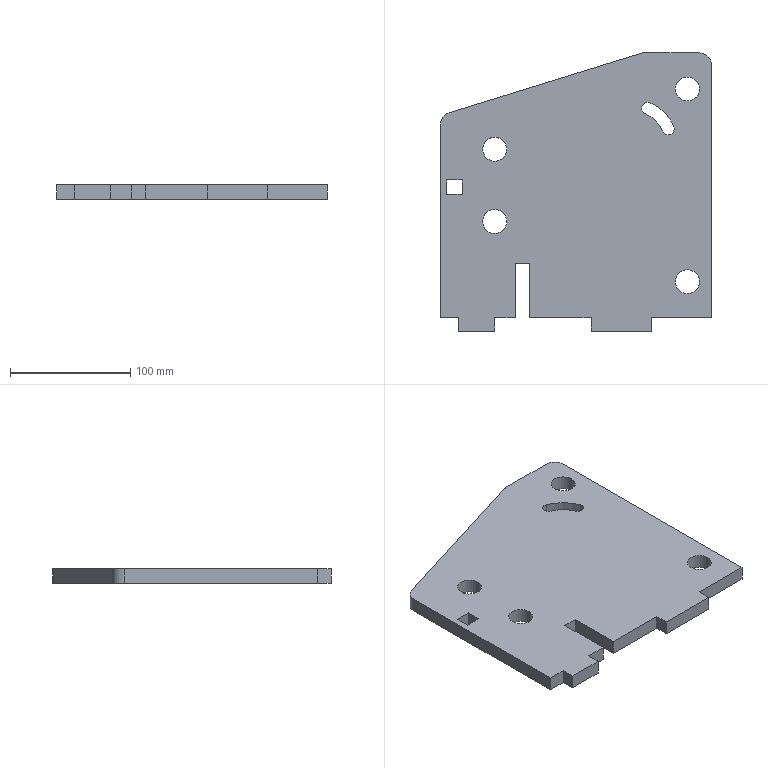Part | SolidWorks | features Fillet 1, FlatPattern 1, SMBaseFlange 1, SheetMetal 1 | 1 solid | 39 faces | box 225 x 231 x 12 mm | volume 524877 mm3 | plane 23 | cylinder 16 | commonest cylinder face diameters 20 x11 10 x3 49 x1 69 x1
STEP:
#1=CARTESIAN_POINT('',(148.788,68.669,12.));
#2=VERTEX_POINT('',#1);
#3=CARTESIAN_POINT('',(142.,64.,12.));
#4=VERTEX_POINT('',#3);
#5=CARTESIAN_POINT('',(147.,64.,12.));
#6=DIRECTION('',(0.,0.,1.));
#7=DIRECTION('',(1.,0.,0.));
#8=AXIS2_PLACEMENT_3D('',#5,#6,#7);
#9=CIRCLE('',#8,5.);
#10=EDGE_CURVE('',#2,#4,#9,.T.);
#11=ORIENTED_EDGE('',*,*,#10,.T.);
#12=CARTESIAN_POINT('',(142.,64.,0.));
#13=VERTEX_POINT('',#12);
#14=CARTESIAN_POINT('',(142.,64.,12.));
#15=DIRECTION('',(0.,0.,-1.));
#16=VECTOR('',#15,1000.);
#17=LINE('',#14,#16);
#18=EDGE_CURVE('',#4,#13,#17,.T.);
#19=ORIENTED_EDGE('',*,*,#18,.T.);
#20=CARTESIAN_POINT('',(148.788,68.669,0.));
#21=VERTEX_POINT('',#20);
#22=CARTESIAN_POINT('',(147.,64.,0.));
#23=DIRECTION('',(0.,0.,1.));
#24=DIRECTION('',(1.,0.,0.));
#25=AXIS2_PLACEMENT_3D('',#22,#23,#24);
#26=CIRCLE('',#25,5.);
#27=EDGE_CURVE('',#21,#13,#26,.T.);
#28=ORIENTED_EDGE('',*,*,#27,.F.);
#29=CARTESIAN_POINT('',(148.788,68.669,12.));
#30=DIRECTION('',(0.,0.,-1.));
#31=VECTOR('',#30,1000.);
#32=LINE('',#29,#31);
#33=EDGE_CURVE('',#2,#21,#32,.T.);
#34=ORIENTED_EDGE('',*,*,#33,.F.);
#35=EDGE_LOOP('',(#11,#19,#28,#34));
#36=FACE_OUTER_BOUND('',#35,.T.);
#37=CARTESIAN_POINT('',(147.,64.,12.));
#38=DIRECTION('',(0.,0.,-1.));
#39=DIRECTION('',(-1.,0.,0.));
#40=AXIS2_PLACEMENT_3D('',#37,#38,#39);
#41=CYLINDRICAL_SURFACE('',#40,5.);
#42=ADVANCED_FACE('',(#36),#41,.F.);
#43=CARTESIAN_POINT('',(170.,80.,12.));
#44=VERTEX_POINT('',#43);
#45=CARTESIAN_POINT('',(190.,80.,12.));
#46=VERTEX_POINT('',#45);
#47=CARTESIAN_POINT('',(180.,80.,12.));
#48=DIRECTION('',(0.,0.,1.));
#49=DIRECTION('',(1.,0.,0.));
#50=AXIS2_PLACEMENT_3D('',#47,#48,#49);
#51=CIRCLE('',#50,10.);
#52=EDGE_CURVE('',#44,#46,#51,.T.);
#53=ORIENTED_EDGE('',*,*,#52,.T.);
#54=CARTESIAN_POINT('',(190.,80.,0.));
#55=VERTEX_POINT('',#54);
#56=CARTESIAN_POINT('',(190.,80.,12.));
#57=DIRECTION('',(0.,0.,-1.));
#58=VECTOR('',#57,1000.);
#59=LINE('',#56,#58);
#60=EDGE_CURVE('',#46,#55,#59,.T.);
#61=ORIENTED_EDGE('',*,*,#60,.T.);
#62=CARTESIAN_POINT('',(170.,80.,0.));
#63=VERTEX_POINT('',#62);
#64=CARTESIAN_POINT('',(180.,80.,0.));
#65=DIRECTION('',(0.,0.,1.));
#66=DIRECTION('',(1.,0.,0.));
#67=AXIS2_PLACEMENT_3D('',#64,#65,#66);
#68=CIRCLE('',#67,10.);
#69=EDGE_CURVE('',#63,#55,#68,.T.);
#70=ORIENTED_EDGE('',*,*,#69,.F.);
#71=CARTESIAN_POINT('',(170.,80.,12.));
#72=DIRECTION('',(0.,0.,-1.));
#73=VECTOR('',#72,1000.);
#74=LINE('',#71,#73);
#75=EDGE_CURVE('',#44,#63,#74,.T.);
#76=ORIENTED_EDGE('',*,*,#75,.F.);
#77=EDGE_LOOP('',(#53,#61,#70,#76));
#78=FACE_OUTER_BOUND('',#77,.T.);
#79=CARTESIAN_POINT('',(180.,80.,12.));
#80=DIRECTION('',(0.,0.,-1.));
#81=DIRECTION('',(-1.,0.,0.));
#82=AXIS2_PLACEMENT_3D('',#79,#80,#81);
#83=CYLINDRICAL_SURFACE('',#82,10.);
#84=ADVANCED_FACE('',(#78),#83,.F.);
#85=CARTESIAN_POINT('',(170.,-80.,12.));
#86=VERTEX_POINT('',#85);
#87=CARTESIAN_POINT('',(190.,-80.,12.));
#88=VERTEX_POINT('',#87);
#89=CARTESIAN_POINT('',(180.,-80.,12.));
#90=DIRECTION('',(0.,0.,1.));
#91=DIRECTION('',(1.,0.,0.));
#92=AXIS2_PLACEMENT_3D('',#89,#90,#91);
#93=CIRCLE('',#92,10.);
#94=EDGE_CURVE('',#86,#88,#93,.T.);
#95=ORIENTED_EDGE('',*,*,#94,.T.);
#96=CARTESIAN_POINT('',(190.,-80.,0.));
#97=VERTEX_POINT('',#96);
#98=CARTESIAN_POINT('',(190.,-80.,12.));
#99=DIRECTION('',(0.,0.,-1.));
#100=VECTOR('',#99,1000.);
#101=LINE('',#98,#100);
#102=EDGE_CURVE('',#88,#97,#101,.T.);
#103=ORIENTED_EDGE('',*,*,#102,.T.);
#104=CARTESIAN_POINT('',(170.,-80.,0.));
#105=VERTEX_POINT('',#104);
#106=CARTESIAN_POINT('',(180.,-80.,0.));
#107=DIRECTION('',(0.,0.,1.));
#108=DIRECTION('',(1.,0.,0.));
#109=AXIS2_PLACEMENT_3D('',#106,#107,#108);
#110=CIRCLE('',#109,10.);
#111=EDGE_CURVE('',#105,#97,#110,.T.);
#112=ORIENTED_EDGE('',*,*,#111,.F.);
#113=CARTESIAN_POINT('',(170.,-80.,12.));
#114=DIRECTION('',(0.,0.,-1.));
#115=VECTOR('',#114,1000.);
#116=LINE('',#113,#115);
#117=EDGE_CURVE('',#86,#105,#116,.T.);
#118=ORIENTED_EDGE('',*,*,#117,.F.);
#119=EDGE_LOOP('',(#95,#103,#112,#118));
#120=FACE_OUTER_BOUND('',#119,.T.);
#121=CARTESIAN_POINT('',(180.,-80.,12.));
#122=DIRECTION('',(0.,0.,-1.));
#123=DIRECTION('',(-1.,0.,0.));
#124=AXIS2_PLACEMENT_3D('',#121,#122,#123);
#125=CYLINDRICAL_SURFACE('',#124,10.);
#126=ADVANCED_FACE('',(#120),#125,.F.);
#127=CARTESIAN_POINT('',(10.,-30.,12.));
#128=VERTEX_POINT('',#127);
#129=CARTESIAN_POINT('',(30.,-30.,12.));
#130=VERTEX_POINT('',#129);
#131=CARTESIAN_POINT('',(20.,-30.,12.));
#132=DIRECTION('',(0.,0.,1.));
#133=DIRECTION('',(1.,0.,0.));
#134=AXIS2_PLACEMENT_3D('',#131,#132,#133);
#135=CIRCLE('',#134,10.);
#136=EDGE_CURVE('',#128,#130,#135,.T.);
#137=ORIENTED_EDGE('',*,*,#136,.T.);
#138=CARTESIAN_POINT('',(30.,-30.,0.));
#139=VERTEX_POINT('',#138);
#140=CARTESIAN_POINT('',(30.,-30.,12.));
#141=DIRECTION('',(0.,0.,-1.));
#142=VECTOR('',#141,1000.);
#143=LINE('',#140,#142);
#144=EDGE_CURVE('',#130,#139,#143,.T.);
#145=ORIENTED_EDGE('',*,*,#144,.T.);
#146=CARTESIAN_POINT('',(10.,-30.,0.));
#147=VERTEX_POINT('',#146);
#148=CARTESIAN_POINT('',(20.,-30.,0.));
#149=DIRECTION('',(0.,0.,1.));
#150=DIRECTION('',(1.,0.,0.));
#151=AXIS2_PLACEMENT_3D('',#148,#149,#150);
#152=CIRCLE('',#151,10.);
#153=EDGE_CURVE('',#147,#139,#152,.T.);
#154=ORIENTED_EDGE('',*,*,#153,.F.);
#155=CARTESIAN_POINT('',(10.,-30.,12.));
#156=DIRECTION('',(0.,0.,-1.));
#157=VECTOR('',#156,1000.);
#158=LINE('',#155,#157);
#159=EDGE_CURVE('',#128,#147,#158,.T.);
#160=ORIENTED_EDGE('',*,*,#159,.F.);
#161=EDGE_LOOP('',(#137,#145,#154,#160));
#162=FACE_OUTER_BOUND('',#161,.T.);
#163=CARTESIAN_POINT('',(20.,-30.,12.));
#164=DIRECTION('',(0.,0.,-1.));
#165=DIRECTION('',(-1.,0.,0.));
#166=AXIS2_PLACEMENT_3D('',#163,#164,#165);
#167=CYLINDRICAL_SURFACE('',#166,10.);
#168=ADVANCED_FACE('',(#162),#167,.F.);
#169=CARTESIAN_POINT('',(10.,30.,12.));
#170=VERTEX_POINT('',#169);
#171=CARTESIAN_POINT('',(30.,30.,12.));
#172=VERTEX_POINT('',#171);
#173=CARTESIAN_POINT('',(20.,30.,12.));
#174=DIRECTION('',(0.,0.,1.));
#175=DIRECTION('',(1.,0.,0.));
#176=AXIS2_PLACEMENT_3D('',#173,#174,#175);
#177=CIRCLE('',#176,10.);
#178=EDGE_CURVE('',#170,#172,#177,.T.);
#179=ORIENTED_EDGE('',*,*,#178,.T.);
#180=CARTESIAN_POINT('',(30.,30.,0.));
#181=VERTEX_POINT('',#180);
#182=CARTESIAN_POINT('',(30.,30.,12.));
#183=DIRECTION('',(0.,0.,-1.));
#184=VECTOR('',#183,1000.);
#185=LINE('',#182,#184);
#186=EDGE_CURVE('',#172,#181,#185,.T.);
#187=ORIENTED_EDGE('',*,*,#186,.T.);
#188=CARTESIAN_POINT('',(10.,30.,0.));
#189=VERTEX_POINT('',#188);
#190=CARTESIAN_POINT('',(20.,30.,0.));
#191=DIRECTION('',(0.,0.,1.));
#192=DIRECTION('',(1.,0.,0.));
#193=AXIS2_PLACEMENT_3D('',#190,#191,#192);
#194=CIRCLE('',#193,10.);
#195=EDGE_CURVE('',#189,#181,#194,.T.);
#196=ORIENTED_EDGE('',*,*,#195,.F.);
#197=CARTESIAN_POINT('',(10.,30.,12.));
#198=DIRECTION('',(0.,0.,-1.));
#199=VECTOR('',#198,1000.);
#200=LINE('',#197,#199);
#201=EDGE_CURVE('',#170,#189,#200,.T.);
#202=ORIENTED_EDGE('',*,*,#201,.F.);
#203=EDGE_LOOP('',(#179,#187,#196,#202));
#204=FACE_OUTER_BOUND('',#203,.T.);
#205=CARTESIAN_POINT('',(20.,30.,12.));
#206=DIRECTION('',(0.,0.,-1.));
#207=DIRECTION('',(-1.,0.,0.));
#208=AXIS2_PLACEMENT_3D('',#205,#206,#207);
#209=CYLINDRICAL_SURFACE('',#208,10.);
#210=ADVANCED_FACE('',(#204),#209,.F.);
#211=CARTESIAN_POINT('',(-7.,-7.5,12.));
#212=VERTEX_POINT('',#211);
#213=CARTESIAN_POINT('',(-7.,4.5,12.));
#214=VERTEX_POINT('',#213);
#215=CARTESIAN_POINT('',(-7.,4.5,12.));
#216=DIRECTION('',(0.,1.,0.));
#217=VECTOR('',#216,1000.);
#218=LINE('',#215,#217);
#219=EDGE_CURVE('',#212,#214,#218,.T.);
#220=ORIENTED_EDGE('',*,*,#219,.F.);
#221=CARTESIAN_POINT('',(-20.,-7.5,12.));
#222=VERTEX_POINT('',#221);
#223=CARTESIAN_POINT('',(-7.,-7.5,12.));
#224=DIRECTION('',(1.,0.,0.));
#225=VECTOR('',#224,1000.);
#226=LINE('',#223,#225);
#227=EDGE_CURVE('',#222,#212,#226,.T.);
#228=ORIENTED_EDGE('',*,*,#227,.F.);
#229=CARTESIAN_POINT('',(-20.,4.5,12.));
#230=VERTEX_POINT('',#229);
#231=CARTESIAN_POINT('',(-20.,4.5,12.));
#232=DIRECTION('',(0.,-1.,0.));
#233=VECTOR('',#232,1000.);
#234=LINE('',#231,#233);
#235=EDGE_CURVE('',#230,#222,#234,.T.);
#236=ORIENTED_EDGE('',*,*,#235,.F.);
#237=CARTESIAN_POINT('',(-7.,4.5,12.));
#238=DIRECTION('',(-1.,0.,0.));
#239=VECTOR('',#238,1000.);
#240=LINE('',#237,#239);
#241=EDGE_CURVE('',#214,#230,#240,.T.);
#242=ORIENTED_EDGE('',*,*,#241,.F.);
#243=EDGE_LOOP('',(#220,#228,#236,#242));
#244=FACE_BOUND('',#243,.T.);
#245=CARTESIAN_POINT('',(200.,-110.,12.));
#246=VERTEX_POINT('',#245);
#247=CARTESIAN_POINT('',(200.,100.,12.));
#248=VERTEX_POINT('',#247);
#249=CARTESIAN_POINT('',(200.,110.,12.));
#250=DIRECTION('',(0.,1.,0.));
#251=VECTOR('',#250,1000.);
#252=LINE('',#249,#251);
#253=EDGE_CURVE('',#246,#248,#252,.T.);
#254=ORIENTED_EDGE('',*,*,#253,.T.);
#255=CARTESIAN_POINT('',(190.,110.,12.));
#256=VERTEX_POINT('',#255);
#257=CARTESIAN_POINT('',(190.,100.,12.));
#258=DIRECTION('',(0.,0.,1.));
#259=DIRECTION('',(-1.,0.,0.));
#260=AXIS2_PLACEMENT_3D('',#257,#258,#259);
#261=CIRCLE('',#260,10.);
#262=EDGE_CURVE('',#248,#256,#261,.T.);
#263=ORIENTED_EDGE('',*,*,#262,.T.);
#264=CARTESIAN_POINT('',(143.647,110.,12.));
#265=VERTEX_POINT('',#264);
#266=CARTESIAN_POINT('',(142.132,110.,12.));
#267=DIRECTION('',(-1.,0.,0.));
#268=VECTOR('',#267,1000.);
#269=LINE('',#266,#268);
#270=EDGE_CURVE('',#256,#265,#269,.T.);
#271=ORIENTED_EDGE('',*,*,#270,.T.);
#272=CARTESIAN_POINT('',(140.686,109.552,12.));
#273=VERTEX_POINT('',#272);
#274=CARTESIAN_POINT('',(143.647,100.,12.));
#275=DIRECTION('',(0.,0.,1.));
#276=DIRECTION('',(-1.,0.,0.));
#277=AXIS2_PLACEMENT_3D('',#274,#275,#276);
#278=CIRCLE('',#277,10.);
#279=EDGE_CURVE('',#265,#273,#278,.T.);
#280=ORIENTED_EDGE('',*,*,#279,.T.);
#281=CARTESIAN_POINT('',(-17.961,60.371,12.));
#282=VERTEX_POINT('',#281);
#283=CARTESIAN_POINT('',(-25.,58.189,12.));
#284=DIRECTION('',(-0.9552,-0.2961,0.));
#285=VECTOR('',#284,1000.);
#286=LINE('',#283,#285);
#287=EDGE_CURVE('',#273,#282,#286,.T.);
#288=ORIENTED_EDGE('',*,*,#287,.T.);
#289=CARTESIAN_POINT('',(-25.,50.819,12.));
#290=VERTEX_POINT('',#289);
#291=CARTESIAN_POINT('',(-15.,50.819,12.));
#292=DIRECTION('',(0.,0.,1.));
#293=DIRECTION('',(-1.,0.,0.));
#294=AXIS2_PLACEMENT_3D('',#291,#292,#293);
#295=CIRCLE('',#294,10.);
#296=EDGE_CURVE('',#282,#290,#295,.T.);
#297=ORIENTED_EDGE('',*,*,#296,.T.);
#298=CARTESIAN_POINT('',(-25.,-110.,12.));
#299=VERTEX_POINT('',#298);
#300=CARTESIAN_POINT('',(-25.,-110.,12.));
#301=DIRECTION('',(0.,-1.,0.));
#302=VECTOR('',#301,1000.);
#303=LINE('',#300,#302);
#304=EDGE_CURVE('',#290,#299,#303,.T.);
#305=ORIENTED_EDGE('',*,*,#304,.T.);
#306=CARTESIAN_POINT('',(-10.,-110.,12.));
#307=VERTEX_POINT('',#306);
#308=CARTESIAN_POINT('',(-25.,-110.,12.));
#309=DIRECTION('',(1.,0.,0.));
#310=VECTOR('',#309,1000.);
#311=LINE('',#308,#310);
#312=EDGE_CURVE('',#299,#307,#311,.T.);
#313=ORIENTED_EDGE('',*,*,#312,.T.);
#314=CARTESIAN_POINT('',(-10.,-121.,12.));
#315=VERTEX_POINT('',#314);
#316=CARTESIAN_POINT('',(-10.,-110.,12.));
#317=DIRECTION('',(0.,-1.,0.));
#318=VECTOR('',#317,1000.);
#319=LINE('',#316,#318);
#320=EDGE_CURVE('',#307,#315,#319,.T.);
#321=ORIENTED_EDGE('',*,*,#320,.T.);
#322=CARTESIAN_POINT('',(20.,-121.,12.));
#323=VERTEX_POINT('',#322);
#324=CARTESIAN_POINT('',(-10.,-121.,12.));
#325=DIRECTION('',(1.,0.,0.));
#326=VECTOR('',#325,1000.);
#327=LINE('',#324,#326);
#328=EDGE_CURVE('',#315,#323,#327,.T.);
#329=ORIENTED_EDGE('',*,*,#328,.T.);
#330=CARTESIAN_POINT('',(20.,-110.,12.));
#331=VERTEX_POINT('',#330);
#332=CARTESIAN_POINT('',(20.,-121.,12.));
#333=DIRECTION('',(0.,1.,0.));
#334=VECTOR('',#333,1000.);
#335=LINE('',#332,#334);
#336=EDGE_CURVE('',#323,#331,#335,.T.);
#337=ORIENTED_EDGE('',*,*,#336,.T.);
#338=CARTESIAN_POINT('',(37.,-110.,12.));
#339=VERTEX_POINT('',#338);
#340=CARTESIAN_POINT('',(20.,-110.,12.));
#341=DIRECTION('',(1.,0.,0.));
#342=VECTOR('',#341,1000.);
#343=LINE('',#340,#342);
#344=EDGE_CURVE('',#331,#339,#343,.T.);
#345=ORIENTED_EDGE('',*,*,#344,.T.);
#346=CARTESIAN_POINT('',(37.,-65.,12.));
#347=VERTEX_POINT('',#346);
#348=CARTESIAN_POINT('',(37.,-110.,12.));
#349=DIRECTION('',(0.,1.,0.));
#350=VECTOR('',#349,1000.);
#351=LINE('',#348,#350);
#352=EDGE_CURVE('',#339,#347,#351,.T.);
#353=ORIENTED_EDGE('',*,*,#352,.T.);
#354=CARTESIAN_POINT('',(49.,-65.,12.));
#355=VERTEX_POINT('',#354);
#356=CARTESIAN_POINT('',(37.,-65.,12.));
#357=DIRECTION('',(1.,0.,0.));
#358=VECTOR('',#357,1000.);
#359=LINE('',#356,#358);
#360=EDGE_CURVE('',#347,#355,#359,.T.);
#361=ORIENTED_EDGE('',*,*,#360,.T.);
#362=CARTESIAN_POINT('',(49.,-110.,12.));
#363=VERTEX_POINT('',#362);
#364=CARTESIAN_POINT('',(49.,-65.,12.));
#365=DIRECTION('',(0.,-1.,0.));
#366=VECTOR('',#365,1000.);
#367=LINE('',#364,#366);
#368=EDGE_CURVE('',#355,#363,#367,.T.);
#369=ORIENTED_EDGE('',*,*,#368,.T.);
#370=CARTESIAN_POINT('',(100.,-110.,12.));
#371=VERTEX_POINT('',#370);
#372=CARTESIAN_POINT('',(49.,-110.,12.));
#373=DIRECTION('',(1.,0.,0.));
#374=VECTOR('',#373,1000.);
#375=LINE('',#372,#374);
#376=EDGE_CURVE('',#363,#371,#375,.T.);
#377=ORIENTED_EDGE('',*,*,#376,.T.);
#378=CARTESIAN_POINT('',(100.,-121.,12.));
#379=VERTEX_POINT('',#378);
#380=CARTESIAN_POINT('',(100.,-110.,12.));
#381=DIRECTION('',(0.,-1.,0.));
#382=VECTOR('',#381,1000.);
#383=LINE('',#380,#382);
#384=EDGE_CURVE('',#371,#379,#383,.T.);
#385=ORIENTED_EDGE('',*,*,#384,.T.);
#386=CARTESIAN_POINT('',(150.,-121.,12.));
#387=VERTEX_POINT('',#386);
#388=CARTESIAN_POINT('',(100.,-121.,12.));
#389=DIRECTION('',(1.,0.,0.));
#390=VECTOR('',#389,1000.);
#391=LINE('',#388,#390);
#392=EDGE_CURVE('',#379,#387,#391,.T.);
#393=ORIENTED_EDGE('',*,*,#392,.T.);
#394=CARTESIAN_POINT('',(150.,-110.,12.));
#395=VERTEX_POINT('',#394);
#396=CARTESIAN_POINT('',(150.,-121.,12.));
#397=DIRECTION('',(0.,1.,0.));
#398=VECTOR('',#397,1000.);
#399=LINE('',#396,#398);
#400=EDGE_CURVE('',#387,#395,#399,.T.);
#401=ORIENTED_EDGE('',*,*,#400,.T.);
#402=CARTESIAN_POINT('',(150.,-110.,12.));
#403=DIRECTION('',(1.,0.,0.));
#404=VECTOR('',#403,1000.);
#405=LINE('',#402,#404);
#406=EDGE_CURVE('',#395,#246,#405,.T.);
#407=ORIENTED_EDGE('',*,*,#406,.T.);
#408=EDGE_LOOP('',(#254,#263,#271,#280,#288,#297,#305,#313,#321,#329,#337,#345,#353,#361,#369,#377,#385,#393,#401,#407));
#409=FACE_OUTER_BOUND('',#408,.T.);
#410=ORIENTED_EDGE('',*,*,#178,.F.);
#411=CARTESIAN_POINT('',(20.,30.,12.));
#412=DIRECTION('',(0.,0.,1.));
#413=DIRECTION('',(1.,0.,0.));
#414=AXIS2_PLACEMENT_3D('',#411,#412,#413);
#415=CIRCLE('',#414,10.);
#416=EDGE_CURVE('',#172,#170,#415,.T.);
#417=ORIENTED_EDGE('',*,*,#416,.F.);
#418=EDGE_LOOP('',(#410,#417));
#419=FACE_BOUND('',#418,.T.);
#420=ORIENTED_EDGE('',*,*,#136,.F.);
#421=CARTESIAN_POINT('',(20.,-30.,12.));
#422=DIRECTION('',(0.,0.,1.));
#423=DIRECTION('',(1.,0.,0.));
#424=AXIS2_PLACEMENT_3D('',#421,#422,#423);
#425=CIRCLE('',#424,10.);
#426=EDGE_CURVE('',#130,#128,#425,.T.);
#427=ORIENTED_EDGE('',*,*,#426,.F.);
#428=EDGE_LOOP('',(#420,#427));
#429=FACE_BOUND('',#428,.T.);
#430=ORIENTED_EDGE('',*,*,#94,.F.);
#431=CARTESIAN_POINT('',(180.,-80.,12.));
#432=DIRECTION('',(0.,0.,1.));
#433=DIRECTION('',(1.,0.,0.));
#434=AXIS2_PLACEMENT_3D('',#431,#432,#433);
#435=CIRCLE('',#434,10.);
#436=EDGE_CURVE('',#88,#86,#435,.T.);
#437=ORIENTED_EDGE('',*,*,#436,.F.);
#438=EDGE_LOOP('',(#430,#437));
#439=FACE_BOUND('',#438,.T.);
#440=ORIENTED_EDGE('',*,*,#52,.F.);
#441=CARTESIAN_POINT('',(180.,80.,12.));
#442=DIRECTION('',(0.,0.,1.));
#443=DIRECTION('',(1.,0.,0.));
#444=AXIS2_PLACEMENT_3D('',#441,#442,#443);
#445=CIRCLE('',#444,10.);
#446=EDGE_CURVE('',#46,#44,#445,.T.);
#447=ORIENTED_EDGE('',*,*,#446,.F.);
#448=EDGE_LOOP('',(#440,#447));
#449=FACE_BOUND('',#448,.T.);
#450=CARTESIAN_POINT('',(145.212,59.331,12.));
#451=VERTEX_POINT('',#450);
#452=CARTESIAN_POINT('',(159.331,45.212,12.));
#453=VERTEX_POINT('',#452);
#454=CARTESIAN_POINT('',(136.451,36.451,12.));
#455=DIRECTION('',(0.,0.,-1.));
#456=DIRECTION('',(1.,0.,0.));
#457=AXIS2_PLACEMENT_3D('',#454,#455,#456);
#458=CIRCLE('',#457,24.5);
#459=EDGE_CURVE('',#451,#453,#458,.T.);
#460=ORIENTED_EDGE('',*,*,#459,.F.);
#461=CARTESIAN_POINT('',(147.,64.,12.));
#462=DIRECTION('',(0.,0.,1.));
#463=DIRECTION('',(1.,0.,0.));
#464=AXIS2_PLACEMENT_3D('',#461,#462,#463);
#465=CIRCLE('',#464,5.);
#466=EDGE_CURVE('',#4,#451,#465,.T.);
#467=ORIENTED_EDGE('',*,*,#466,.F.);
#468=ORIENTED_EDGE('',*,*,#10,.F.);
#469=CARTESIAN_POINT('',(168.669,48.788,12.));
#470=VERTEX_POINT('',#469);
#471=CARTESIAN_POINT('',(136.451,36.451,12.));
#472=DIRECTION('',(0.,0.,1.));
#473=DIRECTION('',(1.,0.,0.));
#474=AXIS2_PLACEMENT_3D('',#471,#472,#473);
#475=CIRCLE('',#474,34.5);
#476=EDGE_CURVE('',#470,#2,#475,.T.);
#477=ORIENTED_EDGE('',*,*,#476,.F.);
#478=CARTESIAN_POINT('',(164.,47.,12.));
#479=DIRECTION('',(0.,0.,1.));
#480=DIRECTION('',(1.,0.,0.));
#481=AXIS2_PLACEMENT_3D('',#478,#479,#480);
#482=CIRCLE('',#481,5.);
#483=EDGE_CURVE('',#453,#470,#482,.T.);
#484=ORIENTED_EDGE('',*,*,#483,.F.);
#485=EDGE_LOOP('',(#460,#467,#468,#477,#484));
#486=FACE_BOUND('',#485,.T.);
#487=CARTESIAN_POINT('',(0.,0.,12.));
#488=DIRECTION('',(0.,0.,-1.));
#489=DIRECTION('',(-1.,0.,0.));
#490=AXIS2_PLACEMENT_3D('',#487,#488,#489);
#491=PLANE('',#490);
#492=ADVANCED_FACE('',(#244,#409,#419,#429,#439,#449,#486),#491,.F.);
#493=ORIENTED_EDGE('',*,*,#111,.T.);
#494=CARTESIAN_POINT('',(180.,-80.,0.));
#495=DIRECTION('',(0.,0.,1.));
#496=DIRECTION('',(1.,0.,0.));
#497=AXIS2_PLACEMENT_3D('',#494,#495,#496);
#498=CIRCLE('',#497,10.);
#499=EDGE_CURVE('',#97,#105,#498,.T.);
#500=ORIENTED_EDGE('',*,*,#499,.T.);
#501=EDGE_LOOP('',(#493,#500));
#502=FACE_BOUND('',#501,.T.);
#503=ORIENTED_EDGE('',*,*,#195,.T.);
#504=CARTESIAN_POINT('',(20.,30.,0.));
#505=DIRECTION('',(0.,0.,1.));
#506=DIRECTION('',(1.,0.,0.));
#507=AXIS2_PLACEMENT_3D('',#504,#505,#506);
#508=CIRCLE('',#507,10.);
#509=EDGE_CURVE('',#181,#189,#508,.T.);
#510=ORIENTED_EDGE('',*,*,#509,.T.);
#511=EDGE_LOOP('',(#503,#510));
#512=FACE_BOUND('',#511,.T.);
#513=CARTESIAN_POINT('',(190.,110.,0.));
#514=VERTEX_POINT('',#513);
#515=CARTESIAN_POINT('',(143.647,110.,0.));
#516=VERTEX_POINT('',#515);
#517=CARTESIAN_POINT('',(142.132,110.,0.));
#518=DIRECTION('',(-1.,0.,0.));
#519=VECTOR('',#518,1000.);
#520=LINE('',#517,#519);
#521=EDGE_CURVE('',#514,#516,#520,.T.);
#522=ORIENTED_EDGE('',*,*,#521,.F.);
#523=CARTESIAN_POINT('',(200.,100.,0.));
#524=VERTEX_POINT('',#523);
#525=CARTESIAN_POINT('',(190.,100.,0.));
#526=DIRECTION('',(0.,0.,-1.));
#527=DIRECTION('',(-1.,0.,0.));
#528=AXIS2_PLACEMENT_3D('',#525,#526,#527);
#529=CIRCLE('',#528,10.);
#530=EDGE_CURVE('',#514,#524,#529,.T.);
#531=ORIENTED_EDGE('',*,*,#530,.T.);
#532=CARTESIAN_POINT('',(200.,-110.,0.));
#533=VERTEX_POINT('',#532);
#534=CARTESIAN_POINT('',(200.,110.,0.));
#535=DIRECTION('',(0.,1.,0.));
#536=VECTOR('',#535,1000.);
#537=LINE('',#534,#536);
#538=EDGE_CURVE('',#533,#524,#537,.T.);
#539=ORIENTED_EDGE('',*,*,#538,.F.);
#540=CARTESIAN_POINT('',(150.,-110.,0.));
#541=VERTEX_POINT('',#540);
#542=CARTESIAN_POINT('',(150.,-110.,0.));
#543=DIRECTION('',(1.,0.,0.));
#544=VECTOR('',#543,1000.);
#545=LINE('',#542,#544);
#546=EDGE_CURVE('',#541,#533,#545,.T.);
#547=ORIENTED_EDGE('',*,*,#546,.F.);
#548=CARTESIAN_POINT('',(150.,-121.,0.));
#549=VERTEX_POINT('',#548);
#550=CARTESIAN_POINT('',(150.,-121.,0.));
#551=DIRECTION('',(0.,1.,0.));
#552=VECTOR('',#551,1000.);
#553=LINE('',#550,#552);
#554=EDGE_CURVE('',#549,#541,#553,.T.);
#555=ORIENTED_EDGE('',*,*,#554,.F.);
#556=CARTESIAN_POINT('',(100.,-121.,0.));
#557=VERTEX_POINT('',#556);
#558=CARTESIAN_POINT('',(100.,-121.,0.));
#559=DIRECTION('',(1.,0.,0.));
#560=VECTOR('',#559,1000.);
#561=LINE('',#558,#560);
#562=EDGE_CURVE('',#557,#549,#561,.T.);
#563=ORIENTED_EDGE('',*,*,#562,.F.);
#564=CARTESIAN_POINT('',(100.,-110.,0.));
#565=VERTEX_POINT('',#564);
#566=CARTESIAN_POINT('',(100.,-110.,0.));
#567=DIRECTION('',(0.,-1.,0.));
#568=VECTOR('',#567,1000.);
#569=LINE('',#566,#568);
#570=EDGE_CURVE('',#565,#557,#569,.T.);
#571=ORIENTED_EDGE('',*,*,#570,.F.);
#572=CARTESIAN_POINT('',(49.,-110.,0.));
#573=VERTEX_POINT('',#572);
#574=CARTESIAN_POINT('',(49.,-110.,0.));
#575=DIRECTION('',(1.,0.,0.));
#576=VECTOR('',#575,1000.);
#577=LINE('',#574,#576);
#578=EDGE_CURVE('',#573,#565,#577,.T.);
#579=ORIENTED_EDGE('',*,*,#578,.F.);
#580=CARTESIAN_POINT('',(49.,-65.,0.));
#581=VERTEX_POINT('',#580);
#582=CARTESIAN_POINT('',(49.,-65.,0.));
#583=DIRECTION('',(0.,-1.,0.));
#584=VECTOR('',#583,1000.);
#585=LINE('',#582,#584);
#586=EDGE_CURVE('',#581,#573,#585,.T.);
#587=ORIENTED_EDGE('',*,*,#586,.F.);
#588=CARTESIAN_POINT('',(37.,-65.,0.));
#589=VERTEX_POINT('',#588);
#590=CARTESIAN_POINT('',(37.,-65.,0.));
#591=DIRECTION('',(1.,0.,0.));
#592=VECTOR('',#591,1000.);
#593=LINE('',#590,#592);
#594=EDGE_CURVE('',#589,#581,#593,.T.);
#595=ORIENTED_EDGE('',*,*,#594,.F.);
#596=CARTESIAN_POINT('',(37.,-110.,0.));
#597=VERTEX_POINT('',#596);
#598=CARTESIAN_POINT('',(37.,-110.,0.));
#599=DIRECTION('',(0.,1.,0.));
#600=VECTOR('',#599,1000.);
#601=LINE('',#598,#600);
#602=EDGE_CURVE('',#597,#589,#601,.T.);
#603=ORIENTED_EDGE('',*,*,#602,.F.);
#604=CARTESIAN_POINT('',(20.,-110.,0.));
#605=VERTEX_POINT('',#604);
#606=CARTESIAN_POINT('',(20.,-110.,0.));
#607=DIRECTION('',(1.,0.,0.));
#608=VECTOR('',#607,1000.);
#609=LINE('',#606,#608);
#610=EDGE_CURVE('',#605,#597,#609,.T.);
#611=ORIENTED_EDGE('',*,*,#610,.F.);
#612=CARTESIAN_POINT('',(20.,-121.,0.));
#613=VERTEX_POINT('',#612);
#614=CARTESIAN_POINT('',(20.,-121.,0.));
#615=DIRECTION('',(0.,1.,0.));
#616=VECTOR('',#615,1000.);
#617=LINE('',#614,#616);
#618=EDGE_CURVE('',#613,#605,#617,.T.);
#619=ORIENTED_EDGE('',*,*,#618,.F.);
#620=CARTESIAN_POINT('',(-10.,-121.,0.));
#621=VERTEX_POINT('',#620);
#622=CARTESIAN_POINT('',(-10.,-121.,0.));
#623=DIRECTION('',(1.,0.,0.));
#624=VECTOR('',#623,1000.);
#625=LINE('',#622,#624);
#626=EDGE_CURVE('',#621,#613,#625,.T.);
#627=ORIENTED_EDGE('',*,*,#626,.F.);
#628=CARTESIAN_POINT('',(-10.,-110.,0.));
#629=VERTEX_POINT('',#628);
#630=CARTESIAN_POINT('',(-10.,-110.,0.));
#631=DIRECTION('',(0.,-1.,0.));
#632=VECTOR('',#631,1000.);
#633=LINE('',#630,#632);
#634=EDGE_CURVE('',#629,#621,#633,.T.);
#635=ORIENTED_EDGE('',*,*,#634,.F.);
#636=CARTESIAN_POINT('',(-25.,-110.,0.));
#637=VERTEX_POINT('',#636);
#638=CARTESIAN_POINT('',(-25.,-110.,0.));
#639=DIRECTION('',(1.,0.,0.));
#640=VECTOR('',#639,1000.);
#641=LINE('',#638,#640);
#642=EDGE_CURVE('',#637,#629,#641,.T.);
#643=ORIENTED_EDGE('',*,*,#642,.F.);
#644=CARTESIAN_POINT('',(-25.,50.819,0.));
#645=VERTEX_POINT('',#644);
#646=CARTESIAN_POINT('',(-25.,-110.,0.));
#647=DIRECTION('',(0.,-1.,0.));
#648=VECTOR('',#647,1000.);
#649=LINE('',#646,#648);
#650=EDGE_CURVE('',#645,#637,#649,.T.);
#651=ORIENTED_EDGE('',*,*,#650,.F.);
#652=CARTESIAN_POINT('',(-17.961,60.371,0.));
#653=VERTEX_POINT('',#652);
#654=CARTESIAN_POINT('',(-15.,50.819,0.));
#655=DIRECTION('',(0.,0.,-1.));
#656=DIRECTION('',(-1.,0.,0.));
#657=AXIS2_PLACEMENT_3D('',#654,#655,#656);
#658=CIRCLE('',#657,10.);
#659=EDGE_CURVE('',#645,#653,#658,.T.);
#660=ORIENTED_EDGE('',*,*,#659,.T.);
#661=CARTESIAN_POINT('',(140.686,109.552,0.));
#662=VERTEX_POINT('',#661);
#663=CARTESIAN_POINT('',(-25.,58.189,0.));
#664=DIRECTION('',(-0.9552,-0.2961,0.));
#665=VECTOR('',#664,1000.);
#666=LINE('',#663,#665);
#667=EDGE_CURVE('',#662,#653,#666,.T.);
#668=ORIENTED_EDGE('',*,*,#667,.F.);
#669=CARTESIAN_POINT('',(143.647,100.,0.));
#670=DIRECTION('',(0.,0.,-1.));
#671=DIRECTION('',(-1.,0.,0.));
#672=AXIS2_PLACEMENT_3D('',#669,#670,#671);
#673=CIRCLE('',#672,10.);
#674=EDGE_CURVE('',#662,#516,#673,.T.);
#675=ORIENTED_EDGE('',*,*,#674,.T.);
#676=EDGE_LOOP('',(#522,#531,#539,#547,#555,#563,#571,#579,#587,#595,#603,#611,#619,#627,#635,#643,#651,#660,#668,#675));
#677=FACE_OUTER_BOUND('',#676,.T.);
#678=ORIENTED_EDGE('',*,*,#153,.T.);
#679=CARTESIAN_POINT('',(20.,-30.,0.));
#680=DIRECTION('',(0.,0.,1.));
#681=DIRECTION('',(1.,0.,0.));
#682=AXIS2_PLACEMENT_3D('',#679,#680,#681);
#683=CIRCLE('',#682,10.);
#684=EDGE_CURVE('',#139,#147,#683,.T.);
#685=ORIENTED_EDGE('',*,*,#684,.T.);
#686=EDGE_LOOP('',(#678,#685));
#687=FACE_BOUND('',#686,.T.);
#688=ORIENTED_EDGE('',*,*,#69,.T.);
#689=CARTESIAN_POINT('',(180.,80.,0.));
#690=DIRECTION('',(0.,0.,1.));
#691=DIRECTION('',(1.,0.,0.));
#692=AXIS2_PLACEMENT_3D('',#689,#690,#691);
#693=CIRCLE('',#692,10.);
#694=EDGE_CURVE('',#55,#63,#693,.T.);
#695=ORIENTED_EDGE('',*,*,#694,.T.);
#696=EDGE_LOOP('',(#688,#695));
#697=FACE_BOUND('',#696,.T.);
#698=CARTESIAN_POINT('',(-20.,-7.5,0.));
#699=VERTEX_POINT('',#698);
#700=CARTESIAN_POINT('',(-7.,-7.5,0.));
#701=VERTEX_POINT('',#700);
#702=CARTESIAN_POINT('',(-7.,-7.5,0.));
#703=DIRECTION('',(1.,0.,0.));
#704=VECTOR('',#703,1000.);
#705=LINE('',#702,#704);
#706=EDGE_CURVE('',#699,#701,#705,.T.);
#707=ORIENTED_EDGE('',*,*,#706,.T.);
#708=CARTESIAN_POINT('',(-7.,4.5,0.));
#709=VERTEX_POINT('',#708);
#710=CARTESIAN_POINT('',(-7.,4.5,0.));
#711=DIRECTION('',(0.,1.,0.));
#712=VECTOR('',#711,1000.);
#713=LINE('',#710,#712);
#714=EDGE_CURVE('',#701,#709,#713,.T.);
#715=ORIENTED_EDGE('',*,*,#714,.T.);
#716=CARTESIAN_POINT('',(-20.,4.5,0.));
#717=VERTEX_POINT('',#716);
#718=CARTESIAN_POINT('',(-7.,4.5,0.));
#719=DIRECTION('',(-1.,0.,0.));
#720=VECTOR('',#719,1000.);
#721=LINE('',#718,#720);
#722=EDGE_CURVE('',#709,#717,#721,.T.);
#723=ORIENTED_EDGE('',*,*,#722,.T.);
#724=CARTESIAN_POINT('',(-20.,4.5,0.));
#725=DIRECTION('',(0.,-1.,0.));
#726=VECTOR('',#725,1000.);
#727=LINE('',#724,#726);
#728=EDGE_CURVE('',#717,#699,#727,.T.);
#729=ORIENTED_EDGE('',*,*,#728,.T.);
#730=EDGE_LOOP('',(#707,#715,#723,#729));
#731=FACE_BOUND('',#730,.T.);
#732=ORIENTED_EDGE('',*,*,#27,.T.);
#733=CARTESIAN_POINT('',(145.212,59.331,0.));
#734=VERTEX_POINT('',#733);
#735=CARTESIAN_POINT('',(147.,64.,0.));
#736=DIRECTION('',(0.,0.,1.));
#737=DIRECTION('',(1.,0.,0.));
#738=AXIS2_PLACEMENT_3D('',#735,#736,#737);
#739=CIRCLE('',#738,5.);
#740=EDGE_CURVE('',#13,#734,#739,.T.);
#741=ORIENTED_EDGE('',*,*,#740,.T.);
#742=CARTESIAN_POINT('',(159.331,45.212,0.));
#743=VERTEX_POINT('',#742);
#744=CARTESIAN_POINT('',(136.451,36.451,0.));
#745=DIRECTION('',(0.,0.,-1.));
#746=DIRECTION('',(1.,0.,0.));
#747=AXIS2_PLACEMENT_3D('',#744,#745,#746);
#748=CIRCLE('',#747,24.5);
#749=EDGE_CURVE('',#734,#743,#748,.T.);
#750=ORIENTED_EDGE('',*,*,#749,.T.);
#751=CARTESIAN_POINT('',(168.669,48.788,0.));
#752=VERTEX_POINT('',#751);
#753=CARTESIAN_POINT('',(164.,47.,0.));
#754=DIRECTION('',(0.,0.,1.));
#755=DIRECTION('',(1.,0.,0.));
#756=AXIS2_PLACEMENT_3D('',#753,#754,#755);
#757=CIRCLE('',#756,5.);
#758=EDGE_CURVE('',#743,#752,#757,.T.);
#759=ORIENTED_EDGE('',*,*,#758,.T.);
#760=CARTESIAN_POINT('',(136.451,36.451,0.));
#761=DIRECTION('',(0.,0.,1.));
#762=DIRECTION('',(1.,0.,0.));
#763=AXIS2_PLACEMENT_3D('',#760,#761,#762);
#764=CIRCLE('',#763,34.5);
#765=EDGE_CURVE('',#752,#21,#764,.T.);
#766=ORIENTED_EDGE('',*,*,#765,.T.);
#767=EDGE_LOOP('',(#732,#741,#750,#759,#766));
#768=FACE_BOUND('',#767,.T.);
#769=CARTESIAN_POINT('',(0.,0.,0.));
#770=DIRECTION('',(0.,0.,-1.));
#771=DIRECTION('',(-1.,0.,0.));
#772=AXIS2_PLACEMENT_3D('',#769,#770,#771);
#773=PLANE('',#772);
#774=ADVANCED_FACE('',(#502,#512,#677,#687,#697,#731,#768),#773,.T.);
#775=ORIENTED_EDGE('',*,*,#546,.T.);
#776=CARTESIAN_POINT('',(200.,-110.,12.));
#777=DIRECTION('',(0.,0.,-1.));
#778=VECTOR('',#777,1000.);
#779=LINE('',#776,#778);
#780=EDGE_CURVE('',#246,#533,#779,.T.);
#781=ORIENTED_EDGE('',*,*,#780,.F.);
#782=ORIENTED_EDGE('',*,*,#406,.F.);
#783=CARTESIAN_POINT('',(150.,-110.,12.));
#784=DIRECTION('',(0.,0.,-1.));
#785=VECTOR('',#784,1000.);
#786=LINE('',#783,#785);
#787=EDGE_CURVE('',#395,#541,#786,.T.);
#788=ORIENTED_EDGE('',*,*,#787,.T.);
#789=EDGE_LOOP('',(#775,#781,#782,#788));
#790=FACE_OUTER_BOUND('',#789,.T.);
#791=CARTESIAN_POINT('',(150.,-110.,12.));
#792=DIRECTION('',(0.,1.,0.));
#793=DIRECTION('',(0.,0.,1.));
#794=AXIS2_PLACEMENT_3D('',#791,#792,#793);
#795=PLANE('',#794);
#796=ADVANCED_FACE('',(#790),#795,.F.);
#797=ORIENTED_EDGE('',*,*,#538,.T.);
#798=CARTESIAN_POINT('',(200.,100.,12.));
#799=DIRECTION('',(0.,0.,1.));
#800=VECTOR('',#799,1000.);
#801=LINE('',#798,#800);
#802=EDGE_CURVE('',#524,#248,#801,.T.);
#803=ORIENTED_EDGE('',*,*,#802,.T.);
#804=ORIENTED_EDGE('',*,*,#253,.F.);
#805=ORIENTED_EDGE('',*,*,#780,.T.);
#806=EDGE_LOOP('',(#797,#803,#804,#805));
#807=FACE_OUTER_BOUND('',#806,.T.);
#808=CARTESIAN_POINT('',(200.,110.,12.));
#809=DIRECTION('',(-1.,0.,0.));
#810=DIRECTION('',(0.,0.,1.));
#811=AXIS2_PLACEMENT_3D('',#808,#809,#810);
#812=PLANE('',#811);
#813=ADVANCED_FACE('',(#807),#812,.F.);
#814=ORIENTED_EDGE('',*,*,#270,.F.);
#815=CARTESIAN_POINT('',(190.,110.,12.));
#816=DIRECTION('',(0.,0.,-1.));
#817=VECTOR('',#816,1000.);
#818=LINE('',#815,#817);
#819=EDGE_CURVE('',#256,#514,#818,.T.);
#820=ORIENTED_EDGE('',*,*,#819,.T.);
#821=ORIENTED_EDGE('',*,*,#521,.T.);
#822=CARTESIAN_POINT('',(143.647,110.,12.));
#823=DIRECTION('',(0.,0.,1.));
#824=VECTOR('',#823,1000.);
#825=LINE('',#822,#824);
#826=EDGE_CURVE('',#516,#265,#825,.T.);
#827=ORIENTED_EDGE('',*,*,#826,.T.);
#828=EDGE_LOOP('',(#814,#820,#821,#827));
#829=FACE_OUTER_BOUND('',#828,.T.);
#830=CARTESIAN_POINT('',(142.132,110.,12.));
#831=DIRECTION('',(0.,-1.,0.));
#832=DIRECTION('',(0.,0.,-1.));
#833=AXIS2_PLACEMENT_3D('',#830,#831,#832);
#834=PLANE('',#833);
#835=ADVANCED_FACE('',(#829),#834,.F.);
#836=ORIENTED_EDGE('',*,*,#287,.F.);
#837=CARTESIAN_POINT('',(140.686,109.552,12.));
#838=DIRECTION('',(0.,0.,-1.));
#839=VECTOR('',#838,1000.);
#840=LINE('',#837,#839);
#841=EDGE_CURVE('',#273,#662,#840,.T.);
#842=ORIENTED_EDGE('',*,*,#841,.T.);
#843=ORIENTED_EDGE('',*,*,#667,.T.);
#844=CARTESIAN_POINT('',(-17.961,60.371,12.));
#845=DIRECTION('',(0.,0.,1.));
#846=VECTOR('',#845,1000.);
#847=LINE('',#844,#846);
#848=EDGE_CURVE('',#653,#282,#847,.T.);
#849=ORIENTED_EDGE('',*,*,#848,.T.);
#850=EDGE_LOOP('',(#836,#842,#843,#849));
#851=FACE_OUTER_BOUND('',#850,.T.);
#852=CARTESIAN_POINT('',(-25.,58.189,12.));
#853=DIRECTION('',(0.2961,-0.9552,0.));
#854=DIRECTION('',(0.9552,0.2961,0.));
#855=AXIS2_PLACEMENT_3D('',#852,#853,#854);
#856=PLANE('',#855);
#857=ADVANCED_FACE('',(#851),#856,.F.);
#858=ORIENTED_EDGE('',*,*,#304,.F.);
#859=CARTESIAN_POINT('',(-25.,50.819,12.));
#860=DIRECTION('',(0.,0.,-1.));
#861=VECTOR('',#860,1000.);
#862=LINE('',#859,#861);
#863=EDGE_CURVE('',#290,#645,#862,.T.);
#864=ORIENTED_EDGE('',*,*,#863,.T.);
#865=ORIENTED_EDGE('',*,*,#650,.T.);
#866=CARTESIAN_POINT('',(-25.,-110.,12.));
#867=DIRECTION('',(0.,0.,-1.));
#868=VECTOR('',#867,1000.);
#869=LINE('',#866,#868);
#870=EDGE_CURVE('',#299,#637,#869,.T.);
#871=ORIENTED_EDGE('',*,*,#870,.F.);
#872=EDGE_LOOP('',(#858,#864,#865,#871));
#873=FACE_OUTER_BOUND('',#872,.T.);
#874=CARTESIAN_POINT('',(-25.,-110.,12.));
#875=DIRECTION('',(1.,0.,0.));
#876=DIRECTION('',(0.,1.,0.));
#877=AXIS2_PLACEMENT_3D('',#874,#875,#876);
#878=PLANE('',#877);
#879=ADVANCED_FACE('',(#873),#878,.F.);
#880=ORIENTED_EDGE('',*,*,#642,.T.);
#881=CARTESIAN_POINT('',(-10.,-110.,12.));
#882=DIRECTION('',(0.,0.,-1.));
#883=VECTOR('',#882,1000.);
#884=LINE('',#881,#883);
#885=EDGE_CURVE('',#307,#629,#884,.T.);
#886=ORIENTED_EDGE('',*,*,#885,.F.);
#887=ORIENTED_EDGE('',*,*,#312,.F.);
#888=ORIENTED_EDGE('',*,*,#870,.T.);
#889=EDGE_LOOP('',(#880,#886,#887,#888));
#890=FACE_OUTER_BOUND('',#889,.T.);
#891=CARTESIAN_POINT('',(-25.,-110.,12.));
#892=DIRECTION('',(0.,1.,0.));
#893=DIRECTION('',(0.,0.,1.));
#894=AXIS2_PLACEMENT_3D('',#891,#892,#893);
#895=PLANE('',#894);
#896=ADVANCED_FACE('',(#890),#895,.F.);
#897=ORIENTED_EDGE('',*,*,#634,.T.);
#898=CARTESIAN_POINT('',(-10.,-121.,12.));
#899=DIRECTION('',(0.,0.,-1.));
#900=VECTOR('',#899,1000.);
#901=LINE('',#898,#900);
#902=EDGE_CURVE('',#315,#621,#901,.T.);
#903=ORIENTED_EDGE('',*,*,#902,.F.);
#904=ORIENTED_EDGE('',*,*,#320,.F.);
#905=ORIENTED_EDGE('',*,*,#885,.T.);
#906=EDGE_LOOP('',(#897,#903,#904,#905));
#907=FACE_OUTER_BOUND('',#906,.T.);
#908=CARTESIAN_POINT('',(-10.,-110.,12.));
#909=DIRECTION('',(1.,0.,0.));
#910=DIRECTION('',(0.,1.,0.));
#911=AXIS2_PLACEMENT_3D('',#908,#909,#910);
#912=PLANE('',#911);
#913=ADVANCED_FACE('',(#907),#912,.F.);
#914=ORIENTED_EDGE('',*,*,#626,.T.);
#915=CARTESIAN_POINT('',(20.,-121.,12.));
#916=DIRECTION('',(0.,0.,-1.));
#917=VECTOR('',#916,1000.);
#918=LINE('',#915,#917);
#919=EDGE_CURVE('',#323,#613,#918,.T.);
#920=ORIENTED_EDGE('',*,*,#919,.F.);
#921=ORIENTED_EDGE('',*,*,#328,.F.);
#922=ORIENTED_EDGE('',*,*,#902,.T.);
#923=EDGE_LOOP('',(#914,#920,#921,#922));
#924=FACE_OUTER_BOUND('',#923,.T.);
#925=CARTESIAN_POINT('',(-10.,-121.,12.));
#926=DIRECTION('',(0.,1.,0.));
#927=DIRECTION('',(0.,0.,1.));
#928=AXIS2_PLACEMENT_3D('',#925,#926,#927);
#929=PLANE('',#928);
#930=ADVANCED_FACE('',(#924),#929,.F.);
#931=ORIENTED_EDGE('',*,*,#618,.T.);
#932=CARTESIAN_POINT('',(20.,-110.,12.));
#933=DIRECTION('',(0.,0.,-1.));
#934=VECTOR('',#933,1000.);
#935=LINE('',#932,#934);
#936=EDGE_CURVE('',#331,#605,#935,.T.);
#937=ORIENTED_EDGE('',*,*,#936,.F.);
#938=ORIENTED_EDGE('',*,*,#336,.F.);
#939=ORIENTED_EDGE('',*,*,#919,.T.);
#940=EDGE_LOOP('',(#931,#937,#938,#939));
#941=FACE_OUTER_BOUND('',#940,.T.);
#942=CARTESIAN_POINT('',(20.,-121.,12.));
#943=DIRECTION('',(-1.,0.,0.));
#944=DIRECTION('',(0.,0.,1.));
#945=AXIS2_PLACEMENT_3D('',#942,#943,#944);
#946=PLANE('',#945);
#947=ADVANCED_FACE('',(#941),#946,.F.);
#948=ORIENTED_EDGE('',*,*,#610,.T.);
#949=CARTESIAN_POINT('',(37.,-110.,12.));
#950=DIRECTION('',(0.,0.,-1.));
#951=VECTOR('',#950,1000.);
#952=LINE('',#949,#951);
#953=EDGE_CURVE('',#339,#597,#952,.T.);
#954=ORIENTED_EDGE('',*,*,#953,.F.);
#955=ORIENTED_EDGE('',*,*,#344,.F.);
#956=ORIENTED_EDGE('',*,*,#936,.T.);
#957=EDGE_LOOP('',(#948,#954,#955,#956));
#958=FACE_OUTER_BOUND('',#957,.T.);
#959=CARTESIAN_POINT('',(20.,-110.,12.));
#960=DIRECTION('',(0.,1.,0.));
#961=DIRECTION('',(-1.,0.,0.));
#962=AXIS2_PLACEMENT_3D('',#959,#960,#961);
#963=PLANE('',#962);
#964=ADVANCED_FACE('',(#958),#963,.F.);
#965=ORIENTED_EDGE('',*,*,#602,.T.);
#966=CARTESIAN_POINT('',(37.,-65.,12.));
#967=DIRECTION('',(0.,0.,-1.));
#968=VECTOR('',#967,1000.);
#969=LINE('',#966,#968);
#970=EDGE_CURVE('',#347,#589,#969,.T.);
#971=ORIENTED_EDGE('',*,*,#970,.F.);
#972=ORIENTED_EDGE('',*,*,#352,.F.);
#973=ORIENTED_EDGE('',*,*,#953,.T.);
#974=EDGE_LOOP('',(#965,#971,#972,#973));
#975=FACE_OUTER_BOUND('',#974,.T.);
#976=CARTESIAN_POINT('',(37.,-110.,12.));
#977=DIRECTION('',(-1.,0.,0.));
#978=DIRECTION('',(0.,-1.,0.));
#979=AXIS2_PLACEMENT_3D('',#976,#977,#978);
#980=PLANE('',#979);
#981=ADVANCED_FACE('',(#975),#980,.F.);
#982=ORIENTED_EDGE('',*,*,#594,.T.);
#983=CARTESIAN_POINT('',(49.,-65.,12.));
#984=DIRECTION('',(0.,0.,-1.));
#985=VECTOR('',#984,1000.);
#986=LINE('',#983,#985);
#987=EDGE_CURVE('',#355,#581,#986,.T.);
#988=ORIENTED_EDGE('',*,*,#987,.F.);
#989=ORIENTED_EDGE('',*,*,#360,.F.);
#990=ORIENTED_EDGE('',*,*,#970,.T.);
#991=EDGE_LOOP('',(#982,#988,#989,#990));
#992=FACE_OUTER_BOUND('',#991,.T.);
#993=CARTESIAN_POINT('',(37.,-65.,12.));
#994=DIRECTION('',(0.,1.,0.));
#995=DIRECTION('',(0.,0.,1.));
#996=AXIS2_PLACEMENT_3D('',#993,#994,#995);
#997=PLANE('',#996);
#998=ADVANCED_FACE('',(#992),#997,.F.);
#999=ORIENTED_EDGE('',*,*,#586,.T.);
#1000=CARTESIAN_POINT('',(49.,-110.,12.));
#1001=DIRECTION('',(0.,0.,-1.));
#1002=VECTOR('',#1001,1000.);
#1003=LINE('',#1000,#1002);
#1004=EDGE_CURVE('',#363,#573,#1003,.T.);
#1005=ORIENTED_EDGE('',*,*,#1004,.F.);
#1006=ORIENTED_EDGE('',*,*,#368,.F.);
#1007=ORIENTED_EDGE('',*,*,#987,.T.);
#1008=EDGE_LOOP('',(#999,#1005,#1006,#1007));
#1009=FACE_OUTER_BOUND('',#1008,.T.);
#1010=CARTESIAN_POINT('',(49.,-65.,12.));
#1011=DIRECTION('',(1.,0.,0.));
#1012=DIRECTION('',(0.,1.,0.));
#1013=AXIS2_PLACEMENT_3D('',#1010,#1011,#1012);
#1014=PLANE('',#1013);
#1015=ADVANCED_FACE('',(#1009),#1014,.F.);
#1016=ORIENTED_EDGE('',*,*,#578,.T.);
#1017=CARTESIAN_POINT('',(100.,-110.,12.));
#1018=DIRECTION('',(0.,0.,-1.));
#1019=VECTOR('',#1018,1000.);
#1020=LINE('',#1017,#1019);
#1021=EDGE_CURVE('',#371,#565,#1020,.T.);
#1022=ORIENTED_EDGE('',*,*,#1021,.F.);
#1023=ORIENTED_EDGE('',*,*,#376,.F.);
#1024=ORIENTED_EDGE('',*,*,#1004,.T.);
#1025=EDGE_LOOP('',(#1016,#1022,#1023,#1024));
#1026=FACE_OUTER_BOUND('',#1025,.T.);
#1027=CARTESIAN_POINT('',(49.,-110.,12.));
#1028=DIRECTION('',(0.,1.,0.));
#1029=DIRECTION('',(-1.,0.,0.));
#1030=AXIS2_PLACEMENT_3D('',#1027,#1028,#1029);
#1031=PLANE('',#1030);
#1032=ADVANCED_FACE('',(#1026),#1031,.F.);
#1033=ORIENTED_EDGE('',*,*,#570,.T.);
#1034=CARTESIAN_POINT('',(100.,-121.,12.));
#1035=DIRECTION('',(0.,0.,-1.));
#1036=VECTOR('',#1035,1000.);
#1037=LINE('',#1034,#1036);
#1038=EDGE_CURVE('',#379,#557,#1037,.T.);
#1039=ORIENTED_EDGE('',*,*,#1038,.F.);
#1040=ORIENTED_EDGE('',*,*,#384,.F.);
#1041=ORIENTED_EDGE('',*,*,#1021,.T.);
#1042=EDGE_LOOP('',(#1033,#1039,#1040,#1041));
#1043=FACE_OUTER_BOUND('',#1042,.T.);
#1044=CARTESIAN_POINT('',(100.,-110.,12.));
#1045=DIRECTION('',(1.,0.,0.));
#1046=DIRECTION('',(0.,0.,-1.));
#1047=AXIS2_PLACEMENT_3D('',#1044,#1045,#1046);
#1048=PLANE('',#1047);
#1049=ADVANCED_FACE('',(#1043),#1048,.F.);
#1050=ORIENTED_EDGE('',*,*,#562,.T.);
#1051=CARTESIAN_POINT('',(150.,-121.,12.));
#1052=DIRECTION('',(0.,0.,-1.));
#1053=VECTOR('',#1052,1000.);
#1054=LINE('',#1051,#1053);
#1055=EDGE_CURVE('',#387,#549,#1054,.T.);
#1056=ORIENTED_EDGE('',*,*,#1055,.F.);
#1057=ORIENTED_EDGE('',*,*,#392,.F.);
#1058=ORIENTED_EDGE('',*,*,#1038,.T.);
#1059=EDGE_LOOP('',(#1050,#1056,#1057,#1058));
#1060=FACE_OUTER_BOUND('',#1059,.T.);
#1061=CARTESIAN_POINT('',(100.,-121.,12.));
#1062=DIRECTION('',(0.,1.,0.));
#1063=DIRECTION('',(0.,0.,1.));
#1064=AXIS2_PLACEMENT_3D('',#1061,#1062,#1063);
#1065=PLANE('',#1064);
#1066=ADVANCED_FACE('',(#1060),#1065,.F.);
#1067=ORIENTED_EDGE('',*,*,#554,.T.);
#1068=ORIENTED_EDGE('',*,*,#787,.F.);
#1069=ORIENTED_EDGE('',*,*,#400,.F.);
#1070=ORIENTED_EDGE('',*,*,#1055,.T.);
#1071=EDGE_LOOP('',(#1067,#1068,#1069,#1070));
#1072=FACE_OUTER_BOUND('',#1071,.T.);
#1073=CARTESIAN_POINT('',(150.,-121.,12.));
#1074=DIRECTION('',(-1.,0.,0.));
#1075=DIRECTION('',(0.,0.,1.));
#1076=AXIS2_PLACEMENT_3D('',#1073,#1074,#1075);
#1077=PLANE('',#1076);
#1078=ADVANCED_FACE('',(#1072),#1077,.F.);
#1079=ORIENTED_EDGE('',*,*,#186,.F.);
#1080=ORIENTED_EDGE('',*,*,#416,.T.);
#1081=ORIENTED_EDGE('',*,*,#201,.T.);
#1082=ORIENTED_EDGE('',*,*,#509,.F.);
#1083=EDGE_LOOP('',(#1079,#1080,#1081,#1082));
#1084=FACE_OUTER_BOUND('',#1083,.T.);
#1085=CARTESIAN_POINT('',(20.,30.,12.));
#1086=DIRECTION('',(0.,0.,-1.));
#1087=DIRECTION('',(-1.,0.,0.));
#1088=AXIS2_PLACEMENT_3D('',#1085,#1086,#1087);
#1089=CYLINDRICAL_SURFACE('',#1088,10.);
#1090=ADVANCED_FACE('',(#1084),#1089,.F.);
#1091=ORIENTED_EDGE('',*,*,#144,.F.);
#1092=ORIENTED_EDGE('',*,*,#426,.T.);
#1093=ORIENTED_EDGE('',*,*,#159,.T.);
#1094=ORIENTED_EDGE('',*,*,#684,.F.);
#1095=EDGE_LOOP('',(#1091,#1092,#1093,#1094));
#1096=FACE_OUTER_BOUND('',#1095,.T.);
#1097=CARTESIAN_POINT('',(20.,-30.,12.));
#1098=DIRECTION('',(0.,0.,-1.));
#1099=DIRECTION('',(-1.,0.,0.));
#1100=AXIS2_PLACEMENT_3D('',#1097,#1098,#1099);
#1101=CYLINDRICAL_SURFACE('',#1100,10.);
#1102=ADVANCED_FACE('',(#1096),#1101,.F.);
#1103=ORIENTED_EDGE('',*,*,#102,.F.);
#1104=ORIENTED_EDGE('',*,*,#436,.T.);
#1105=ORIENTED_EDGE('',*,*,#117,.T.);
#1106=ORIENTED_EDGE('',*,*,#499,.F.);
#1107=EDGE_LOOP('',(#1103,#1104,#1105,#1106));
#1108=FACE_OUTER_BOUND('',#1107,.T.);
#1109=CARTESIAN_POINT('',(180.,-80.,12.));
#1110=DIRECTION('',(0.,0.,-1.));
#1111=DIRECTION('',(-1.,0.,0.));
#1112=AXIS2_PLACEMENT_3D('',#1109,#1110,#1111);
#1113=CYLINDRICAL_SURFACE('',#1112,10.);
#1114=ADVANCED_FACE('',(#1108),#1113,.F.);
#1115=ORIENTED_EDGE('',*,*,#60,.F.);
#1116=ORIENTED_EDGE('',*,*,#446,.T.);
#1117=ORIENTED_EDGE('',*,*,#75,.T.);
#1118=ORIENTED_EDGE('',*,*,#694,.F.);
#1119=EDGE_LOOP('',(#1115,#1116,#1117,#1118));
#1120=FACE_OUTER_BOUND('',#1119,.T.);
#1121=CARTESIAN_POINT('',(180.,80.,12.));
#1122=DIRECTION('',(0.,0.,-1.));
#1123=DIRECTION('',(-1.,0.,0.));
#1124=AXIS2_PLACEMENT_3D('',#1121,#1122,#1123);
#1125=CYLINDRICAL_SURFACE('',#1124,10.);
#1126=ADVANCED_FACE('',(#1120),#1125,.F.);
#1127=ORIENTED_EDGE('',*,*,#714,.F.);
#1128=CARTESIAN_POINT('',(-7.,-7.5,12.));
#1129=DIRECTION('',(0.,0.,-1.));
#1130=VECTOR('',#1129,1000.);
#1131=LINE('',#1128,#1130);
#1132=EDGE_CURVE('',#212,#701,#1131,.T.);
#1133=ORIENTED_EDGE('',*,*,#1132,.F.);
#1134=ORIENTED_EDGE('',*,*,#219,.T.);
#1135=CARTESIAN_POINT('',(-7.,4.5,12.));
#1136=DIRECTION('',(0.,0.,-1.));
#1137=VECTOR('',#1136,1000.);
#1138=LINE('',#1135,#1137);
#1139=EDGE_CURVE('',#214,#709,#1138,.T.);
#1140=ORIENTED_EDGE('',*,*,#1139,.T.);
#1141=EDGE_LOOP('',(#1127,#1133,#1134,#1140));
#1142=FACE_OUTER_BOUND('',#1141,.T.);
#1143=CARTESIAN_POINT('',(-7.,4.5,12.));
#1144=DIRECTION('',(-1.,0.,0.));
#1145=DIRECTION('',(0.,0.,1.));
#1146=AXIS2_PLACEMENT_3D('',#1143,#1144,#1145);
#1147=PLANE('',#1146);
#1148=ADVANCED_FACE('',(#1142),#1147,.T.);
#1149=ORIENTED_EDGE('',*,*,#722,.F.);
#1150=ORIENTED_EDGE('',*,*,#1139,.F.);
#1151=ORIENTED_EDGE('',*,*,#241,.T.);
#1152=CARTESIAN_POINT('',(-20.,4.5,12.));
#1153=DIRECTION('',(0.,0.,-1.));
#1154=VECTOR('',#1153,1000.);
#1155=LINE('',#1152,#1154);
#1156=EDGE_CURVE('',#230,#717,#1155,.T.);
#1157=ORIENTED_EDGE('',*,*,#1156,.T.);
#1158=EDGE_LOOP('',(#1149,#1150,#1151,#1157));
#1159=FACE_OUTER_BOUND('',#1158,.T.);
#1160=CARTESIAN_POINT('',(-7.,4.5,12.));
#1161=DIRECTION('',(0.,-1.,0.));
#1162=DIRECTION('',(0.,0.,-1.));
#1163=AXIS2_PLACEMENT_3D('',#1160,#1161,#1162);
#1164=PLANE('',#1163);
#1165=ADVANCED_FACE('',(#1159),#1164,.T.);
#1166=ORIENTED_EDGE('',*,*,#728,.F.);
#1167=ORIENTED_EDGE('',*,*,#1156,.F.);
#1168=ORIENTED_EDGE('',*,*,#235,.T.);
#1169=CARTESIAN_POINT('',(-20.,-7.5,12.));
#1170=DIRECTION('',(0.,0.,-1.));
#1171=VECTOR('',#1170,1000.);
#1172=LINE('',#1169,#1171);
#1173=EDGE_CURVE('',#222,#699,#1172,.T.);
#1174=ORIENTED_EDGE('',*,*,#1173,.T.);
#1175=EDGE_LOOP('',(#1166,#1167,#1168,#1174));
#1176=FACE_OUTER_BOUND('',#1175,.T.);
#1177=CARTESIAN_POINT('',(-20.,4.5,12.));
#1178=DIRECTION('',(1.,0.,0.));
#1179=DIRECTION('',(0.,0.,-1.));
#1180=AXIS2_PLACEMENT_3D('',#1177,#1178,#1179);
#1181=PLANE('',#1180);
#1182=ADVANCED_FACE('',(#1176),#1181,.T.);
#1183=ORIENTED_EDGE('',*,*,#706,.F.);
#1184=ORIENTED_EDGE('',*,*,#1173,.F.);
#1185=ORIENTED_EDGE('',*,*,#227,.T.);
#1186=ORIENTED_EDGE('',*,*,#1132,.T.);
#1187=EDGE_LOOP('',(#1183,#1184,#1185,#1186));
#1188=FACE_OUTER_BOUND('',#1187,.T.);
#1189=CARTESIAN_POINT('',(-7.,-7.5,12.));
#1190=DIRECTION('',(0.,1.,0.));
#1191=DIRECTION('',(0.,0.,1.));
#1192=AXIS2_PLACEMENT_3D('',#1189,#1190,#1191);
#1193=PLANE('',#1192);
#1194=ADVANCED_FACE('',(#1188),#1193,.T.);
#1195=ORIENTED_EDGE('',*,*,#749,.F.);
#1196=CARTESIAN_POINT('',(145.212,59.331,12.));
#1197=DIRECTION('',(0.,0.,-1.));
#1198=VECTOR('',#1197,1000.);
#1199=LINE('',#1196,#1198);
#1200=EDGE_CURVE('',#451,#734,#1199,.T.);
#1201=ORIENTED_EDGE('',*,*,#1200,.F.);
#1202=ORIENTED_EDGE('',*,*,#459,.T.);
#1203=CARTESIAN_POINT('',(159.331,45.212,12.));
#1204=DIRECTION('',(0.,0.,-1.));
#1205=VECTOR('',#1204,1000.);
#1206=LINE('',#1203,#1205);
#1207=EDGE_CURVE('',#453,#743,#1206,.T.);
#1208=ORIENTED_EDGE('',*,*,#1207,.T.);
#1209=EDGE_LOOP('',(#1195,#1201,#1202,#1208));
#1210=FACE_OUTER_BOUND('',#1209,.T.);
#1211=CARTESIAN_POINT('',(136.451,36.451,12.));
#1212=DIRECTION('',(0.,0.,-1.));
#1213=DIRECTION('',(-1.,0.,0.));
#1214=AXIS2_PLACEMENT_3D('',#1211,#1212,#1213);
#1215=CYLINDRICAL_SURFACE('',#1214,24.5);
#1216=ADVANCED_FACE('',(#1210),#1215,.T.);
#1217=ORIENTED_EDGE('',*,*,#758,.F.);
#1218=ORIENTED_EDGE('',*,*,#1207,.F.);
#1219=ORIENTED_EDGE('',*,*,#483,.T.);
#1220=CARTESIAN_POINT('',(168.669,48.788,12.));
#1221=DIRECTION('',(0.,0.,-1.));
#1222=VECTOR('',#1221,1000.);
#1223=LINE('',#1220,#1222);
#1224=EDGE_CURVE('',#470,#752,#1223,.T.);
#1225=ORIENTED_EDGE('',*,*,#1224,.T.);
#1226=EDGE_LOOP('',(#1217,#1218,#1219,#1225));
#1227=FACE_OUTER_BOUND('',#1226,.T.);
#1228=CARTESIAN_POINT('',(164.,47.,12.));
#1229=DIRECTION('',(0.,0.,-1.));
#1230=DIRECTION('',(-1.,0.,0.));
#1231=AXIS2_PLACEMENT_3D('',#1228,#1229,#1230);
#1232=CYLINDRICAL_SURFACE('',#1231,5.);
#1233=ADVANCED_FACE('',(#1227),#1232,.F.);
#1234=ORIENTED_EDGE('',*,*,#765,.F.);
#1235=ORIENTED_EDGE('',*,*,#1224,.F.);
#1236=ORIENTED_EDGE('',*,*,#476,.T.);
#1237=ORIENTED_EDGE('',*,*,#33,.T.);
#1238=EDGE_LOOP('',(#1234,#1235,#1236,#1237));
#1239=FACE_OUTER_BOUND('',#1238,.T.);
#1240=CARTESIAN_POINT('',(136.451,36.451,12.));
#1241=DIRECTION('',(0.,0.,-1.));
#1242=DIRECTION('',(-1.,0.,0.));
#1243=AXIS2_PLACEMENT_3D('',#1240,#1241,#1242);
#1244=CYLINDRICAL_SURFACE('',#1243,34.5);
#1245=ADVANCED_FACE('',(#1239),#1244,.F.);
#1246=ORIENTED_EDGE('',*,*,#18,.F.);
#1247=ORIENTED_EDGE('',*,*,#466,.T.);
#1248=ORIENTED_EDGE('',*,*,#1200,.T.);
#1249=ORIENTED_EDGE('',*,*,#740,.F.);
#1250=EDGE_LOOP('',(#1246,#1247,#1248,#1249));
#1251=FACE_OUTER_BOUND('',#1250,.T.);
#1252=CARTESIAN_POINT('',(147.,64.,12.));
#1253=DIRECTION('',(0.,0.,-1.));
#1254=DIRECTION('',(-1.,0.,0.));
#1255=AXIS2_PLACEMENT_3D('',#1252,#1253,#1254);
#1256=CYLINDRICAL_SURFACE('',#1255,5.);
#1257=ADVANCED_FACE('',(#1251),#1256,.F.);
#1258=ORIENTED_EDGE('',*,*,#262,.F.);
#1259=ORIENTED_EDGE('',*,*,#802,.F.);
#1260=ORIENTED_EDGE('',*,*,#530,.F.);
#1261=ORIENTED_EDGE('',*,*,#819,.F.);
#1262=EDGE_LOOP('',(#1258,#1259,#1260,#1261));
#1263=FACE_OUTER_BOUND('',#1262,.T.);
#1264=CARTESIAN_POINT('',(190.,100.,12.));
#1265=DIRECTION('',(0.,0.,-1.));
#1266=DIRECTION('',(-1.,0.,0.));
#1267=AXIS2_PLACEMENT_3D('',#1264,#1265,#1266);
#1268=CYLINDRICAL_SURFACE('',#1267,10.);
#1269=ADVANCED_FACE('',(#1263),#1268,.T.);
#1270=ORIENTED_EDGE('',*,*,#279,.F.);
#1271=ORIENTED_EDGE('',*,*,#826,.F.);
#1272=ORIENTED_EDGE('',*,*,#674,.F.);
#1273=ORIENTED_EDGE('',*,*,#841,.F.);
#1274=EDGE_LOOP('',(#1270,#1271,#1272,#1273));
#1275=FACE_OUTER_BOUND('',#1274,.T.);
#1276=CARTESIAN_POINT('',(143.647,100.,12.));
#1277=DIRECTION('',(0.,0.,-1.));
#1278=DIRECTION('',(-1.,0.,0.));
#1279=AXIS2_PLACEMENT_3D('',#1276,#1277,#1278);
#1280=CYLINDRICAL_SURFACE('',#1279,10.);
#1281=ADVANCED_FACE('',(#1275),#1280,.T.);
#1282=ORIENTED_EDGE('',*,*,#296,.F.);
#1283=ORIENTED_EDGE('',*,*,#848,.F.);
#1284=ORIENTED_EDGE('',*,*,#659,.F.);
#1285=ORIENTED_EDGE('',*,*,#863,.F.);
#1286=EDGE_LOOP('',(#1282,#1283,#1284,#1285));
#1287=FACE_OUTER_BOUND('',#1286,.T.);
#1288=CARTESIAN_POINT('',(-15.,50.819,12.));
#1289=DIRECTION('',(0.,0.,-1.));
#1290=DIRECTION('',(-1.,0.,0.));
#1291=AXIS2_PLACEMENT_3D('',#1288,#1289,#1290);
#1292=CYLINDRICAL_SURFACE('',#1291,10.);
#1293=ADVANCED_FACE('',(#1287),#1292,.T.);
#1294=CLOSED_SHELL('',(#42,#84,#126,#168,#210,#492,#774,#796,#813,#835,#857,#879,#896,#913,#930,#947,#964,#981,#998,#1015,#1032,#1049,#1066,#1078,#1090,#1102,#1114,#1126,#1148,#1165,#1182,#1194,#1216,#1233,#1245,#1257,#1269,#1281,#1293));
#1295=MANIFOLD_SOLID_BREP('',#1294);
#1296=CARTESIAN_POINT('',(0.,0.,0.));
#1297=DIRECTION('',(0.,0.,1.));
#1298=DIRECTION('',(1.,0.,0.));
#1299=AXIS2_PLACEMENT_3D('',#1296,#1297,#1298);
#1300=(LENGTH_UNIT()NAMED_UNIT(*)SI_UNIT(.MILLI.,.METRE.));
#1301=UNCERTAINTY_MEASURE_WITH_UNIT(LENGTH_MEASURE(0.00001),#1300,'','');
#1302=(NAMED_UNIT(*)PLANE_ANGLE_UNIT()SI_UNIT($,.RADIAN.));
#1303=(NAMED_UNIT(*)SI_UNIT($,.STERADIAN.)SOLID_ANGLE_UNIT());
#1304=(GEOMETRIC_REPRESENTATION_CONTEXT(3)GLOBAL_UNCERTAINTY_ASSIGNED_CONTEXT((#1301))GLOBAL_UNIT_ASSIGNED_CONTEXT((#1300,#1302,#1303))REPRESENTATION_CONTEXT('',''));
#1305=ADVANCED_BREP_SHAPE_REPRESENTATION('',(#1295,#1299),#1304);